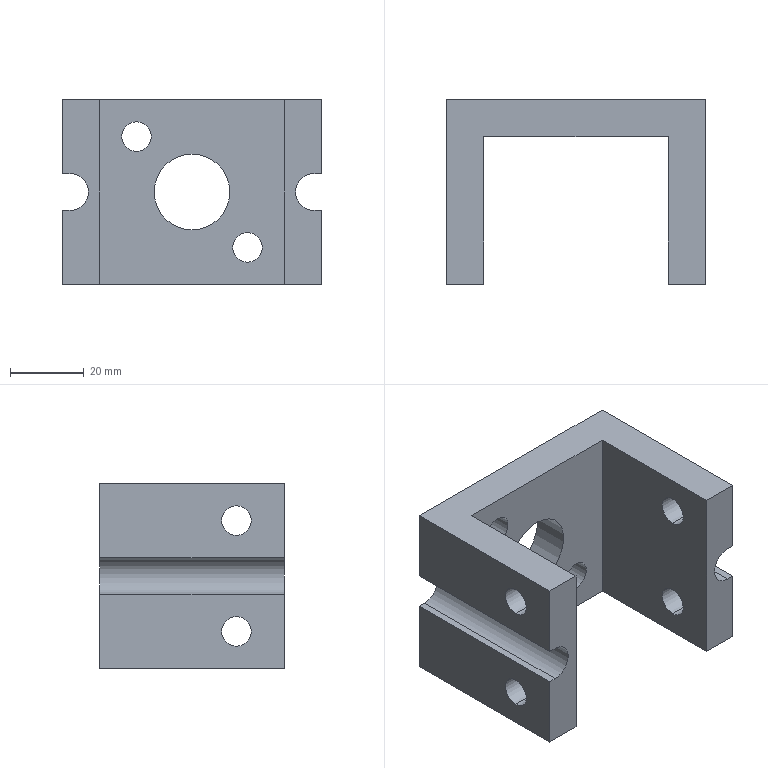Part | STEP file | BCC3 H13_11 | 1 solid | 32 faces | box 70 x 50 x 50 mm | volume 62756 mm3 | cylinder 16 | plane 16 | commonest cylinder face diameters 8 x12 10 x2 20.5 x2